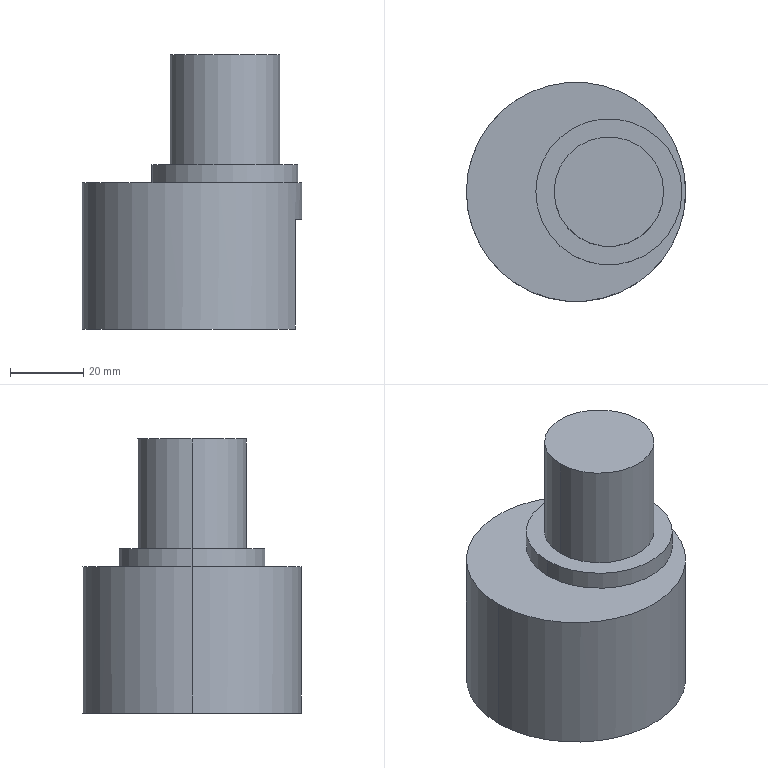Part | SolidWorks | features ICE 3, Extrusion 1, HoleWzd 1 | 1 solid | 17 faces | box 60 x 60 x 75 mm | volume 108504 mm3 | cylinder 10 | plane 7 | commonest cylinder face diameters 10.2 x2 30 x2 36 x2 40 x2 60 x2
STEP:
#1=CARTESIAN_POINT('',(18.,0.,20.1));
#2=VERTEX_POINT('',#1);
#3=CARTESIAN_POINT('',(18.,0.,9.9));
#4=VERTEX_POINT('',#3);
#5=CARTESIAN_POINT('',(18.,0.,20.1));
#6=CARTESIAN_POINT('',(18.,-0.3338,20.1));
#7=CARTESIAN_POINT('',(17.991,-0.668,20.067));
#8=CARTESIAN_POINT('',(17.954,-1.33,19.935));
#9=CARTESIAN_POINT('',(17.927,-1.649,19.837));
#10=CARTESIAN_POINT('',(17.86,-2.264,19.582));
#11=CARTESIAN_POINT('',(17.819,-2.562,19.422));
#12=CARTESIAN_POINT('',(17.731,-3.115,19.052));
#13=CARTESIAN_POINT('',(17.683,-3.37,18.842));
#14=CARTESIAN_POINT('',(17.611,-3.723,18.489));
#15=CARTESIAN_POINT('',(17.587,-3.836,18.365));
#16=CARTESIAN_POINT('',(17.539,-4.047,18.107));
#17=CARTESIAN_POINT('',(17.516,-4.146,17.974));
#18=CARTESIAN_POINT('',(17.449,-4.422,17.562));
#19=CARTESIAN_POINT('',(17.408,-4.58,17.27));
#20=CARTESIAN_POINT('',(17.338,-4.838,16.648));
#21=CARTESIAN_POINT('',(17.31,-4.935,16.328));
#22=CARTESIAN_POINT('',(17.282,-5.033,15.838));
#23=CARTESIAN_POINT('',(17.275,-5.058,15.673));
#24=CARTESIAN_POINT('',(17.265,-5.092,15.339));
#25=CARTESIAN_POINT('',(17.262,-5.1,15.169));
#26=CARTESIAN_POINT('',(17.262,-5.1,14.665));
#27=CARTESIAN_POINT('',(17.272,-5.067,14.332));
#28=CARTESIAN_POINT('',(17.31,-4.937,13.676));
#29=CARTESIAN_POINT('',(17.338,-4.837,13.351));
#30=CARTESIAN_POINT('',(17.408,-4.582,12.736));
#31=CARTESIAN_POINT('',(17.449,-4.426,12.443));
#32=CARTESIAN_POINT('',(17.539,-4.053,11.886));
#33=CARTESIAN_POINT('',(17.587,-3.842,11.629));
#34=CARTESIAN_POINT('',(17.659,-3.491,11.278));
#35=CARTESIAN_POINT('',(17.682,-3.368,11.167));
#36=CARTESIAN_POINT('',(17.73,-3.111,10.956));
#37=CARTESIAN_POINT('',(17.753,-2.976,10.855));
#38=CARTESIAN_POINT('',(17.819,-2.561,10.577));
#39=CARTESIAN_POINT('',(17.859,-2.269,10.42));
#40=CARTESIAN_POINT('',(17.926,-1.654,10.164));
#41=CARTESIAN_POINT('',(17.954,-1.329,10.065));
#42=CARTESIAN_POINT('',(17.99,-0.6722,9.933));
#43=CARTESIAN_POINT('',(18.,-0.3387,9.9));
#44=CARTESIAN_POINT('',(18.,0.,9.9));
#45=B_SPLINE_CURVE_WITH_KNOTS('',3,(#5,#6,#7,#8,#9,#10,#11,#12,#13,#14,#15,#16,#17,#18,#19,#20,#21,#22,#23,#24,#25,#26,#27,#28,#29,#30,#31,#32,#33,#34,#35,#36,#37,#38,#39,#40,#41,#42,#43,#44),.UNSPECIFIED.,.F.,.F.,(4,2,2,2,2,2,2,2,2,2,2,2,2,2,2,2,2,2,2,4),(0.01603,0.01703,0.01803,0.01903,0.02003,0.02053,0.02103,0.02204,0.02304,0.02354,0.02404,0.02504,0.02604,0.02704,0.02804,0.02855,0.02905,0.03005,0.03105,0.03205),.UNSPECIFIED.);
#46=EDGE_CURVE('',#2,#4,#45,.T.);
#47=ORIENTED_EDGE('',*,*,#46,.F.);
#48=CARTESIAN_POINT('',(28.284,0.,20.1));
#49=VERTEX_POINT('',#48);
#50=CARTESIAN_POINT('',(28.284,0.,20.1));
#51=DIRECTION('',(1.,0.,0.));
#52=VECTOR('',#51,1000.);
#53=LINE('',#50,#52);
#54=EDGE_CURVE('',#2,#49,#53,.T.);
#55=ORIENTED_EDGE('',*,*,#54,.T.);
#56=CARTESIAN_POINT('',(28.284,0.,9.9));
#57=VERTEX_POINT('',#56);
#58=CARTESIAN_POINT('',(28.284,0.,15.));
#59=DIRECTION('',(1.,0.,0.));
#60=DIRECTION('',(0.,0.,-1.));
#61=AXIS2_PLACEMENT_3D('',#58,#59,#60);
#62=CIRCLE('',#61,5.1);
#63=EDGE_CURVE('',#49,#57,#62,.T.);
#64=ORIENTED_EDGE('',*,*,#63,.T.);
#65=CARTESIAN_POINT('',(28.284,0.,9.9));
#66=DIRECTION('',(1.,0.,0.));
#67=VECTOR('',#66,1000.);
#68=LINE('',#65,#67);
#69=EDGE_CURVE('',#4,#57,#68,.T.);
#70=ORIENTED_EDGE('',*,*,#69,.F.);
#71=EDGE_LOOP('',(#47,#55,#64,#70));
#72=FACE_OUTER_BOUND('',#71,.T.);
#73=CARTESIAN_POINT('',(28.284,0.,15.));
#74=DIRECTION('',(1.,0.,0.));
#75=DIRECTION('',(0.,0.,-1.));
#76=AXIS2_PLACEMENT_3D('',#73,#74,#75);
#77=CYLINDRICAL_SURFACE('',#76,5.1);
#78=ADVANCED_FACE('',(#72),#77,.F.);
#79=CARTESIAN_POINT('',(18.,0.,30.));
#80=VERTEX_POINT('',#79);
#81=CARTESIAN_POINT('',(-18.,0.,30.));
#82=VERTEX_POINT('',#81);
#83=CARTESIAN_POINT('',(0.,0.,30.));
#84=DIRECTION('',(0.,0.,-1.));
#85=DIRECTION('',(-1.,0.,0.));
#86=AXIS2_PLACEMENT_3D('',#83,#84,#85);
#87=CIRCLE('',#86,18.);
#88=EDGE_CURVE('',#80,#82,#87,.T.);
#89=ORIENTED_EDGE('',*,*,#88,.F.);
#90=CARTESIAN_POINT('',(18.,0.,30.));
#91=DIRECTION('',(0.,0.,-1.));
#92=VECTOR('',#91,1000.);
#93=LINE('',#90,#92);
#94=EDGE_CURVE('',#80,#2,#93,.T.);
#95=ORIENTED_EDGE('',*,*,#94,.T.);
#96=ORIENTED_EDGE('',*,*,#46,.T.);
#97=CARTESIAN_POINT('',(18.,0.,0.));
#98=VERTEX_POINT('',#97);
#99=CARTESIAN_POINT('',(18.,0.,30.));
#100=DIRECTION('',(0.,0.,-1.));
#101=VECTOR('',#100,1000.);
#102=LINE('',#99,#101);
#103=EDGE_CURVE('',#4,#98,#102,.T.);
#104=ORIENTED_EDGE('',*,*,#103,.T.);
#105=CARTESIAN_POINT('',(-18.,0.,0.));
#106=VERTEX_POINT('',#105);
#107=CARTESIAN_POINT('',(0.,0.,0.));
#108=DIRECTION('',(0.,0.,-1.));
#109=DIRECTION('',(-1.,0.,0.));
#110=AXIS2_PLACEMENT_3D('',#107,#108,#109);
#111=CIRCLE('',#110,18.);
#112=EDGE_CURVE('',#98,#106,#111,.T.);
#113=ORIENTED_EDGE('',*,*,#112,.T.);
#114=CARTESIAN_POINT('',(-18.,0.,30.));
#115=DIRECTION('',(0.,0.,-1.));
#116=VECTOR('',#115,1000.);
#117=LINE('',#114,#116);
#118=EDGE_CURVE('',#82,#106,#117,.T.);
#119=ORIENTED_EDGE('',*,*,#118,.F.);
#120=EDGE_LOOP('',(#89,#95,#96,#104,#113,#119));
#121=FACE_OUTER_BOUND('',#120,.T.);
#122=CARTESIAN_POINT('',(0.,0.,30.));
#123=DIRECTION('',(0.,0.,-1.));
#124=DIRECTION('',(-1.,0.,0.));
#125=AXIS2_PLACEMENT_3D('',#122,#123,#124);
#126=CYLINDRICAL_SURFACE('',#125,18.);
#127=ADVANCED_FACE('',(#121),#126,.F.);
#128=CARTESIAN_POINT('',(24.,0.,75.));
#129=VERTEX_POINT('',#128);
#130=CARTESIAN_POINT('',(-6.,0.,75.));
#131=VERTEX_POINT('',#130);
#132=CARTESIAN_POINT('',(9.,0.,75.));
#133=DIRECTION('',(0.,0.,1.));
#134=DIRECTION('',(1.,0.,0.));
#135=AXIS2_PLACEMENT_3D('',#132,#133,#134);
#136=CIRCLE('',#135,15.);
#137=EDGE_CURVE('',#129,#131,#136,.T.);
#138=ORIENTED_EDGE('',*,*,#137,.F.);
#139=CARTESIAN_POINT('',(24.,0.,45.));
#140=VERTEX_POINT('',#139);
#141=CARTESIAN_POINT('',(24.,0.,75.));
#142=DIRECTION('',(0.,0.,-1.));
#143=VECTOR('',#142,1000.);
#144=LINE('',#141,#143);
#145=EDGE_CURVE('',#129,#140,#144,.T.);
#146=ORIENTED_EDGE('',*,*,#145,.T.);
#147=CARTESIAN_POINT('',(-6.,0.,45.));
#148=VERTEX_POINT('',#147);
#149=CARTESIAN_POINT('',(9.,0.,45.));
#150=DIRECTION('',(0.,0.,1.));
#151=DIRECTION('',(1.,0.,0.));
#152=AXIS2_PLACEMENT_3D('',#149,#150,#151);
#153=CIRCLE('',#152,15.);
#154=EDGE_CURVE('',#140,#148,#153,.T.);
#155=ORIENTED_EDGE('',*,*,#154,.T.);
#156=CARTESIAN_POINT('',(-6.,0.,75.));
#157=DIRECTION('',(0.,0.,-1.));
#158=VECTOR('',#157,1000.);
#159=LINE('',#156,#158);
#160=EDGE_CURVE('',#131,#148,#159,.T.);
#161=ORIENTED_EDGE('',*,*,#160,.F.);
#162=EDGE_LOOP('',(#138,#146,#155,#161));
#163=FACE_OUTER_BOUND('',#162,.T.);
#164=CARTESIAN_POINT('',(9.,0.,75.));
#165=DIRECTION('',(0.,0.,-1.));
#166=DIRECTION('',(-1.,0.,0.));
#167=AXIS2_PLACEMENT_3D('',#164,#165,#166);
#168=CYLINDRICAL_SURFACE('',#167,15.);
#169=ADVANCED_FACE('',(#163),#168,.T.);
#170=CARTESIAN_POINT('',(29.,0.,45.));
#171=VERTEX_POINT('',#170);
#172=CARTESIAN_POINT('',(-11.,0.,45.));
#173=VERTEX_POINT('',#172);
#174=CARTESIAN_POINT('',(9.,0.,45.));
#175=DIRECTION('',(0.,0.,1.));
#176=DIRECTION('',(1.,0.,0.));
#177=AXIS2_PLACEMENT_3D('',#174,#175,#176);
#178=CIRCLE('',#177,20.);
#179=EDGE_CURVE('',#171,#173,#178,.T.);
#180=ORIENTED_EDGE('',*,*,#179,.F.);
#181=CARTESIAN_POINT('',(29.,0.,40.));
#182=VERTEX_POINT('',#181);
#183=CARTESIAN_POINT('',(29.,0.,45.));
#184=DIRECTION('',(0.,0.,-1.));
#185=VECTOR('',#184,1000.);
#186=LINE('',#183,#185);
#187=EDGE_CURVE('',#171,#182,#186,.T.);
#188=ORIENTED_EDGE('',*,*,#187,.T.);
#189=CARTESIAN_POINT('',(-11.,0.,40.));
#190=VERTEX_POINT('',#189);
#191=CARTESIAN_POINT('',(9.,0.,40.));
#192=DIRECTION('',(0.,0.,1.));
#193=DIRECTION('',(1.,0.,0.));
#194=AXIS2_PLACEMENT_3D('',#191,#192,#193);
#195=CIRCLE('',#194,20.);
#196=EDGE_CURVE('',#182,#190,#195,.T.);
#197=ORIENTED_EDGE('',*,*,#196,.T.);
#198=CARTESIAN_POINT('',(-11.,0.,45.));
#199=DIRECTION('',(0.,0.,-1.));
#200=VECTOR('',#199,1000.);
#201=LINE('',#198,#200);
#202=EDGE_CURVE('',#173,#190,#201,.T.);
#203=ORIENTED_EDGE('',*,*,#202,.F.);
#204=EDGE_LOOP('',(#180,#188,#197,#203));
#205=FACE_OUTER_BOUND('',#204,.T.);
#206=CARTESIAN_POINT('',(9.,0.,45.));
#207=DIRECTION('',(0.,0.,-1.));
#208=DIRECTION('',(-1.,0.,0.));
#209=AXIS2_PLACEMENT_3D('',#206,#207,#208);
#210=CYLINDRICAL_SURFACE('',#209,20.);
#211=ADVANCED_FACE('',(#205),#210,.T.);
#212=CARTESIAN_POINT('',(30.,0.,40.));
#213=VERTEX_POINT('',#212);
#214=CARTESIAN_POINT('',(-30.,0.,40.));
#215=VERTEX_POINT('',#214);
#216=CARTESIAN_POINT('',(0.,0.,40.));
#217=DIRECTION('',(0.,0.,1.));
#218=DIRECTION('',(1.,0.,0.));
#219=AXIS2_PLACEMENT_3D('',#216,#217,#218);
#220=CIRCLE('',#219,30.);
#221=EDGE_CURVE('',#213,#215,#220,.T.);
#222=ORIENTED_EDGE('',*,*,#221,.F.);
#223=CARTESIAN_POINT('',(30.,0.,30.));
#224=VERTEX_POINT('',#223);
#225=CARTESIAN_POINT('',(30.,0.,40.));
#226=DIRECTION('',(0.,0.,-1.));
#227=VECTOR('',#226,1000.);
#228=LINE('',#225,#227);
#229=EDGE_CURVE('',#213,#224,#228,.T.);
#230=ORIENTED_EDGE('',*,*,#229,.T.);
#231=CARTESIAN_POINT('',(28.284,10.,30.));
#232=VERTEX_POINT('',#231);
#233=CARTESIAN_POINT('',(0.,0.,30.));
#234=DIRECTION('',(0.,0.,1.));
#235=DIRECTION('',(1.,0.,0.));
#236=AXIS2_PLACEMENT_3D('',#233,#234,#235);
#237=CIRCLE('',#236,30.);
#238=EDGE_CURVE('',#224,#232,#237,.T.);
#239=ORIENTED_EDGE('',*,*,#238,.T.);
#240=CARTESIAN_POINT('',(28.284,10.,0.));
#241=VERTEX_POINT('',#240);
#242=CARTESIAN_POINT('',(28.284,10.,30.));
#243=DIRECTION('',(0.,0.,-1.));
#244=VECTOR('',#243,1000.);
#245=LINE('',#242,#244);
#246=EDGE_CURVE('',#232,#241,#245,.T.);
#247=ORIENTED_EDGE('',*,*,#246,.T.);
#248=CARTESIAN_POINT('',(-30.,0.,0.));
#249=VERTEX_POINT('',#248);
#250=CARTESIAN_POINT('',(0.,0.,0.));
#251=DIRECTION('',(0.,0.,1.));
#252=DIRECTION('',(1.,0.,0.));
#253=AXIS2_PLACEMENT_3D('',#250,#251,#252);
#254=CIRCLE('',#253,30.);
#255=EDGE_CURVE('',#241,#249,#254,.T.);
#256=ORIENTED_EDGE('',*,*,#255,.T.);
#257=CARTESIAN_POINT('',(-30.,0.,40.));
#258=DIRECTION('',(0.,0.,-1.));
#259=VECTOR('',#258,1000.);
#260=LINE('',#257,#259);
#261=EDGE_CURVE('',#215,#249,#260,.T.);
#262=ORIENTED_EDGE('',*,*,#261,.F.);
#263=EDGE_LOOP('',(#222,#230,#239,#247,#256,#262));
#264=FACE_OUTER_BOUND('',#263,.T.);
#265=CARTESIAN_POINT('',(0.,0.,40.));
#266=DIRECTION('',(0.,0.,-1.));
#267=DIRECTION('',(-1.,0.,0.));
#268=AXIS2_PLACEMENT_3D('',#265,#266,#267);
#269=CYLINDRICAL_SURFACE('',#268,30.);
#270=ADVANCED_FACE('',(#264),#269,.T.);
#271=CARTESIAN_POINT('',(9.,0.,45.));
#272=DIRECTION('',(0.,0.,1.));
#273=DIRECTION('',(1.,0.,0.));
#274=AXIS2_PLACEMENT_3D('',#271,#272,#273);
#275=CIRCLE('',#274,20.);
#276=EDGE_CURVE('',#173,#171,#275,.T.);
#277=ORIENTED_EDGE('',*,*,#276,.T.);
#278=ORIENTED_EDGE('',*,*,#179,.T.);
#279=EDGE_LOOP('',(#277,#278));
#280=FACE_OUTER_BOUND('',#279,.T.);
#281=CARTESIAN_POINT('',(9.,0.,45.));
#282=DIRECTION('',(0.,0.,1.));
#283=DIRECTION('',(1.,0.,0.));
#284=AXIS2_PLACEMENT_3D('',#281,#282,#283);
#285=CIRCLE('',#284,15.);
#286=EDGE_CURVE('',#148,#140,#285,.T.);
#287=ORIENTED_EDGE('',*,*,#286,.F.);
#288=ORIENTED_EDGE('',*,*,#154,.F.);
#289=EDGE_LOOP('',(#287,#288));
#290=FACE_BOUND('',#289,.T.);
#291=CARTESIAN_POINT('',(9.,0.,45.));
#292=DIRECTION('',(0.,0.,1.));
#293=DIRECTION('',(1.,0.,0.));
#294=AXIS2_PLACEMENT_3D('',#291,#292,#293);
#295=PLANE('',#294);
#296=ADVANCED_FACE('',(#280,#290),#295,.T.);
#297=CARTESIAN_POINT('',(0.,0.,40.));
#298=DIRECTION('',(0.,0.,1.));
#299=DIRECTION('',(1.,0.,0.));
#300=AXIS2_PLACEMENT_3D('',#297,#298,#299);
#301=CIRCLE('',#300,30.);
#302=EDGE_CURVE('',#215,#213,#301,.T.);
#303=ORIENTED_EDGE('',*,*,#302,.T.);
#304=ORIENTED_EDGE('',*,*,#221,.T.);
#305=EDGE_LOOP('',(#303,#304));
#306=FACE_OUTER_BOUND('',#305,.T.);
#307=CARTESIAN_POINT('',(9.,0.,40.));
#308=DIRECTION('',(0.,0.,1.));
#309=DIRECTION('',(1.,0.,0.));
#310=AXIS2_PLACEMENT_3D('',#307,#308,#309);
#311=CIRCLE('',#310,20.);
#312=EDGE_CURVE('',#190,#182,#311,.T.);
#313=ORIENTED_EDGE('',*,*,#312,.F.);
#314=ORIENTED_EDGE('',*,*,#196,.F.);
#315=EDGE_LOOP('',(#313,#314));
#316=FACE_BOUND('',#315,.T.);
#317=CARTESIAN_POINT('',(0.,0.,40.));
#318=DIRECTION('',(0.,0.,1.));
#319=DIRECTION('',(1.,0.,0.));
#320=AXIS2_PLACEMENT_3D('',#317,#318,#319);
#321=PLANE('',#320);
#322=ADVANCED_FACE('',(#306,#316),#321,.T.);
#323=ORIENTED_EDGE('',*,*,#229,.F.);
#324=ORIENTED_EDGE('',*,*,#302,.F.);
#325=ORIENTED_EDGE('',*,*,#261,.T.);
#326=CARTESIAN_POINT('',(28.284,-10.,0.));
#327=VERTEX_POINT('',#326);
#328=CARTESIAN_POINT('',(0.,0.,0.));
#329=DIRECTION('',(0.,0.,1.));
#330=DIRECTION('',(1.,0.,0.));
#331=AXIS2_PLACEMENT_3D('',#328,#329,#330);
#332=CIRCLE('',#331,30.);
#333=EDGE_CURVE('',#249,#327,#332,.T.);
#334=ORIENTED_EDGE('',*,*,#333,.T.);
#335=CARTESIAN_POINT('',(28.284,-10.,30.));
#336=VERTEX_POINT('',#335);
#337=CARTESIAN_POINT('',(28.284,-10.,30.));
#338=DIRECTION('',(0.,0.,-1.));
#339=VECTOR('',#338,1000.);
#340=LINE('',#337,#339);
#341=EDGE_CURVE('',#336,#327,#340,.T.);
#342=ORIENTED_EDGE('',*,*,#341,.F.);
#343=CARTESIAN_POINT('',(0.,0.,30.));
#344=DIRECTION('',(0.,0.,1.));
#345=DIRECTION('',(1.,0.,0.));
#346=AXIS2_PLACEMENT_3D('',#343,#344,#345);
#347=CIRCLE('',#346,30.);
#348=EDGE_CURVE('',#336,#224,#347,.T.);
#349=ORIENTED_EDGE('',*,*,#348,.T.);
#350=EDGE_LOOP('',(#323,#324,#325,#334,#342,#349));
#351=FACE_OUTER_BOUND('',#350,.T.);
#352=CARTESIAN_POINT('',(0.,0.,40.));
#353=DIRECTION('',(0.,0.,-1.));
#354=DIRECTION('',(-1.,0.,0.));
#355=AXIS2_PLACEMENT_3D('',#352,#353,#354);
#356=CYLINDRICAL_SURFACE('',#355,30.);
#357=ADVANCED_FACE('',(#351),#356,.T.);
#358=CARTESIAN_POINT('',(0.,0.,0.));
#359=DIRECTION('',(0.,0.,-1.));
#360=DIRECTION('',(-1.,0.,0.));
#361=AXIS2_PLACEMENT_3D('',#358,#359,#360);
#362=CIRCLE('',#361,18.);
#363=EDGE_CURVE('',#106,#98,#362,.T.);
#364=ORIENTED_EDGE('',*,*,#363,.F.);
#365=ORIENTED_EDGE('',*,*,#112,.F.);
#366=EDGE_LOOP('',(#364,#365));
#367=FACE_BOUND('',#366,.T.);
#368=ORIENTED_EDGE('',*,*,#255,.F.);
#369=CARTESIAN_POINT('',(28.284,10.,0.));
#370=DIRECTION('',(0.,1.,0.));
#371=VECTOR('',#370,1000.);
#372=LINE('',#369,#371);
#373=EDGE_CURVE('',#327,#241,#372,.T.);
#374=ORIENTED_EDGE('',*,*,#373,.F.);
#375=ORIENTED_EDGE('',*,*,#333,.F.);
#376=EDGE_LOOP('',(#368,#374,#375));
#377=FACE_OUTER_BOUND('',#376,.T.);
#378=CARTESIAN_POINT('',(0.,0.,0.));
#379=DIRECTION('',(0.,0.,1.));
#380=DIRECTION('',(1.,0.,0.));
#381=AXIS2_PLACEMENT_3D('',#378,#379,#380);
#382=PLANE('',#381);
#383=ADVANCED_FACE('',(#367,#377),#382,.F.);
#384=ORIENTED_EDGE('',*,*,#187,.F.);
#385=ORIENTED_EDGE('',*,*,#276,.F.);
#386=ORIENTED_EDGE('',*,*,#202,.T.);
#387=ORIENTED_EDGE('',*,*,#312,.T.);
#388=EDGE_LOOP('',(#384,#385,#386,#387));
#389=FACE_OUTER_BOUND('',#388,.T.);
#390=CARTESIAN_POINT('',(9.,0.,45.));
#391=DIRECTION('',(0.,0.,-1.));
#392=DIRECTION('',(-1.,0.,0.));
#393=AXIS2_PLACEMENT_3D('',#390,#391,#392);
#394=CYLINDRICAL_SURFACE('',#393,20.);
#395=ADVANCED_FACE('',(#389),#394,.T.);
#396=ORIENTED_EDGE('',*,*,#145,.F.);
#397=CARTESIAN_POINT('',(9.,0.,75.));
#398=DIRECTION('',(0.,0.,1.));
#399=DIRECTION('',(1.,0.,0.));
#400=AXIS2_PLACEMENT_3D('',#397,#398,#399);
#401=CIRCLE('',#400,15.);
#402=EDGE_CURVE('',#131,#129,#401,.T.);
#403=ORIENTED_EDGE('',*,*,#402,.F.);
#404=ORIENTED_EDGE('',*,*,#160,.T.);
#405=ORIENTED_EDGE('',*,*,#286,.T.);
#406=EDGE_LOOP('',(#396,#403,#404,#405));
#407=FACE_OUTER_BOUND('',#406,.T.);
#408=CARTESIAN_POINT('',(9.,0.,75.));
#409=DIRECTION('',(0.,0.,-1.));
#410=DIRECTION('',(-1.,0.,0.));
#411=AXIS2_PLACEMENT_3D('',#408,#409,#410);
#412=CYLINDRICAL_SURFACE('',#411,15.);
#413=ADVANCED_FACE('',(#407),#412,.T.);
#414=ORIENTED_EDGE('',*,*,#402,.T.);
#415=ORIENTED_EDGE('',*,*,#137,.T.);
#416=EDGE_LOOP('',(#414,#415));
#417=FACE_OUTER_BOUND('',#416,.T.);
#418=CARTESIAN_POINT('',(9.,0.,75.));
#419=DIRECTION('',(0.,0.,1.));
#420=DIRECTION('',(1.,0.,0.));
#421=AXIS2_PLACEMENT_3D('',#418,#419,#420);
#422=PLANE('',#421);
#423=ADVANCED_FACE('',(#417),#422,.T.);
#424=ORIENTED_EDGE('',*,*,#94,.F.);
#425=CARTESIAN_POINT('',(0.,0.,30.));
#426=DIRECTION('',(0.,0.,-1.));
#427=DIRECTION('',(-1.,0.,0.));
#428=AXIS2_PLACEMENT_3D('',#425,#426,#427);
#429=CIRCLE('',#428,18.);
#430=EDGE_CURVE('',#82,#80,#429,.T.);
#431=ORIENTED_EDGE('',*,*,#430,.F.);
#432=ORIENTED_EDGE('',*,*,#118,.T.);
#433=ORIENTED_EDGE('',*,*,#363,.T.);
#434=ORIENTED_EDGE('',*,*,#103,.F.);
#435=CARTESIAN_POINT('',(18.,0.,9.9));
#436=CARTESIAN_POINT('',(18.,0.3388,9.9));
#437=CARTESIAN_POINT('',(17.99,0.6717,9.933));
#438=CARTESIAN_POINT('',(17.954,1.326,10.064));
#439=CARTESIAN_POINT('',(17.927,1.651,10.163));
#440=CARTESIAN_POINT('',(17.859,2.268,10.42));
#441=CARTESIAN_POINT('',(17.819,2.56,10.577));
#442=CARTESIAN_POINT('',(17.731,3.113,10.947));
#443=CARTESIAN_POINT('',(17.683,3.374,11.161));
#444=CARTESIAN_POINT('',(17.587,3.841,11.629));
#445=CARTESIAN_POINT('',(17.539,4.052,11.885));
#446=CARTESIAN_POINT('',(17.449,4.425,12.442));
#447=CARTESIAN_POINT('',(17.408,4.582,12.736));
#448=CARTESIAN_POINT('',(17.356,4.773,13.195));
#449=CARTESIAN_POINT('',(17.34,4.829,13.352));
#450=CARTESIAN_POINT('',(17.313,4.927,13.672));
#451=CARTESIAN_POINT('',(17.301,4.968,13.837));
#452=CARTESIAN_POINT('',(17.272,5.067,14.331));
#453=CARTESIAN_POINT('',(17.262,5.1,14.663));
#454=CARTESIAN_POINT('',(17.262,5.1,15.332));
#455=CARTESIAN_POINT('',(17.272,5.067,15.672));
#456=CARTESIAN_POINT('',(17.31,4.935,16.328));
#457=CARTESIAN_POINT('',(17.338,4.839,16.647));
#458=CARTESIAN_POINT('',(17.408,4.581,17.266));
#459=CARTESIAN_POINT('',(17.449,4.422,17.562));
#460=CARTESIAN_POINT('',(17.539,4.054,18.112));
#461=CARTESIAN_POINT('',(17.587,3.841,18.372));
#462=CARTESIAN_POINT('',(17.683,3.369,18.843));
#463=CARTESIAN_POINT('',(17.731,3.114,19.053));
#464=CARTESIAN_POINT('',(17.819,2.563,19.422));
#465=CARTESIAN_POINT('',(17.86,2.264,19.582));
#466=CARTESIAN_POINT('',(17.927,1.649,19.838));
#467=CARTESIAN_POINT('',(17.954,1.331,19.935));
#468=CARTESIAN_POINT('',(17.981,0.837,20.034));
#469=CARTESIAN_POINT('',(17.988,0.6688,20.059));
#470=CARTESIAN_POINT('',(17.998,0.3341,20.092));
#471=CARTESIAN_POINT('',(18.,0.167,20.1));
#472=CARTESIAN_POINT('',(18.,0.,20.1));
#473=B_SPLINE_CURVE_WITH_KNOTS('',3,(#435,#436,#437,#438,#439,#440,#441,#442,#443,#444,#445,#446,#447,#448,#449,#450,#451,#452,#453,#454,#455,#456,#457,#458,#459,#460,#461,#462,#463,#464,#465,#466,#467,#468,#469,#470,#471,#472),.UNSPECIFIED.,.F.,.F.,(4,2,2,2,2,2,2,2,2,2,2,2,2,2,2,2,2,2,4),(0.,0.001002,0.002003,0.003005,0.004007,0.005009,0.00601,0.006511,0.007012,0.008014,0.009015,0.01002,0.01102,0.01202,0.01302,0.01402,0.01503,0.01553,0.01603),.UNSPECIFIED.);
#474=EDGE_CURVE('',#4,#2,#473,.T.);
#475=ORIENTED_EDGE('',*,*,#474,.T.);
#476=EDGE_LOOP('',(#424,#431,#432,#433,#434,#475));
#477=FACE_OUTER_BOUND('',#476,.T.);
#478=CARTESIAN_POINT('',(0.,0.,30.));
#479=DIRECTION('',(0.,0.,-1.));
#480=DIRECTION('',(-1.,0.,0.));
#481=AXIS2_PLACEMENT_3D('',#478,#479,#480);
#482=CYLINDRICAL_SURFACE('',#481,18.);
#483=ADVANCED_FACE('',(#477),#482,.F.);
#484=ORIENTED_EDGE('',*,*,#430,.T.);
#485=ORIENTED_EDGE('',*,*,#88,.T.);
#486=EDGE_LOOP('',(#484,#485));
#487=FACE_OUTER_BOUND('',#486,.T.);
#488=CARTESIAN_POINT('',(0.,0.,30.));
#489=DIRECTION('',(0.,0.,-1.));
#490=DIRECTION('',(-1.,0.,0.));
#491=AXIS2_PLACEMENT_3D('',#488,#489,#490);
#492=PLANE('',#491);
#493=ADVANCED_FACE('',(#487),#492,.T.);
#494=CARTESIAN_POINT('',(28.284,10.,30.));
#495=DIRECTION('',(0.,1.,0.));
#496=VECTOR('',#495,1000.);
#497=LINE('',#494,#496);
#498=EDGE_CURVE('',#336,#232,#497,.T.);
#499=ORIENTED_EDGE('',*,*,#498,.T.);
#500=ORIENTED_EDGE('',*,*,#238,.F.);
#501=ORIENTED_EDGE('',*,*,#348,.F.);
#502=EDGE_LOOP('',(#499,#500,#501));
#503=FACE_OUTER_BOUND('',#502,.T.);
#504=CARTESIAN_POINT('',(0.,0.,30.));
#505=DIRECTION('',(0.,0.,1.));
#506=DIRECTION('',(1.,0.,0.));
#507=AXIS2_PLACEMENT_3D('',#504,#505,#506);
#508=PLANE('',#507);
#509=ADVANCED_FACE('',(#503),#508,.F.);
#510=CARTESIAN_POINT('',(28.284,0.,15.));
#511=DIRECTION('',(1.,0.,0.));
#512=DIRECTION('',(0.,0.,-1.));
#513=AXIS2_PLACEMENT_3D('',#510,#511,#512);
#514=CIRCLE('',#513,5.1);
#515=EDGE_CURVE('',#57,#49,#514,.T.);
#516=ORIENTED_EDGE('',*,*,#515,.F.);
#517=ORIENTED_EDGE('',*,*,#63,.F.);
#518=EDGE_LOOP('',(#516,#517));
#519=FACE_BOUND('',#518,.T.);
#520=ORIENTED_EDGE('',*,*,#373,.T.);
#521=ORIENTED_EDGE('',*,*,#246,.F.);
#522=ORIENTED_EDGE('',*,*,#498,.F.);
#523=ORIENTED_EDGE('',*,*,#341,.T.);
#524=EDGE_LOOP('',(#520,#521,#522,#523));
#525=FACE_OUTER_BOUND('',#524,.T.);
#526=CARTESIAN_POINT('',(28.284,10.,30.));
#527=DIRECTION('',(-1.,0.,0.));
#528=DIRECTION('',(0.,0.,1.));
#529=AXIS2_PLACEMENT_3D('',#526,#527,#528);
#530=PLANE('',#529);
#531=ADVANCED_FACE('',(#519,#525),#530,.F.);
#532=ORIENTED_EDGE('',*,*,#54,.F.);
#533=ORIENTED_EDGE('',*,*,#474,.F.);
#534=ORIENTED_EDGE('',*,*,#69,.T.);
#535=ORIENTED_EDGE('',*,*,#515,.T.);
#536=EDGE_LOOP('',(#532,#533,#534,#535));
#537=FACE_OUTER_BOUND('',#536,.T.);
#538=CARTESIAN_POINT('',(28.284,0.,15.));
#539=DIRECTION('',(1.,0.,0.));
#540=DIRECTION('',(0.,0.,-1.));
#541=AXIS2_PLACEMENT_3D('',#538,#539,#540);
#542=CYLINDRICAL_SURFACE('',#541,5.1);
#543=ADVANCED_FACE('',(#537),#542,.F.);
#544=CLOSED_SHELL('',(#78,#127,#169,#211,#270,#296,#322,#357,#383,#395,#413,#423,#483,#493,#509,#531,#543));
#545=MANIFOLD_SOLID_BREP('',#544);
#546=CARTESIAN_POINT('',(0.,0.,0.));
#547=DIRECTION('',(0.,0.,1.));
#548=DIRECTION('',(1.,0.,0.));
#549=AXIS2_PLACEMENT_3D('',#546,#547,#548);
#550=(LENGTH_UNIT()NAMED_UNIT(*)SI_UNIT(.MILLI.,.METRE.));
#551=UNCERTAINTY_MEASURE_WITH_UNIT(LENGTH_MEASURE(0.00001),#550,'','');
#552=(NAMED_UNIT(*)PLANE_ANGLE_UNIT()SI_UNIT($,.RADIAN.));
#553=(NAMED_UNIT(*)SI_UNIT($,.STERADIAN.)SOLID_ANGLE_UNIT());
#554=(GEOMETRIC_REPRESENTATION_CONTEXT(3)GLOBAL_UNCERTAINTY_ASSIGNED_CONTEXT((#551))GLOBAL_UNIT_ASSIGNED_CONTEXT((#550,#552,#553))REPRESENTATION_CONTEXT('',''));
#555=ADVANCED_BREP_SHAPE_REPRESENTATION('',(#545,#549),#554);